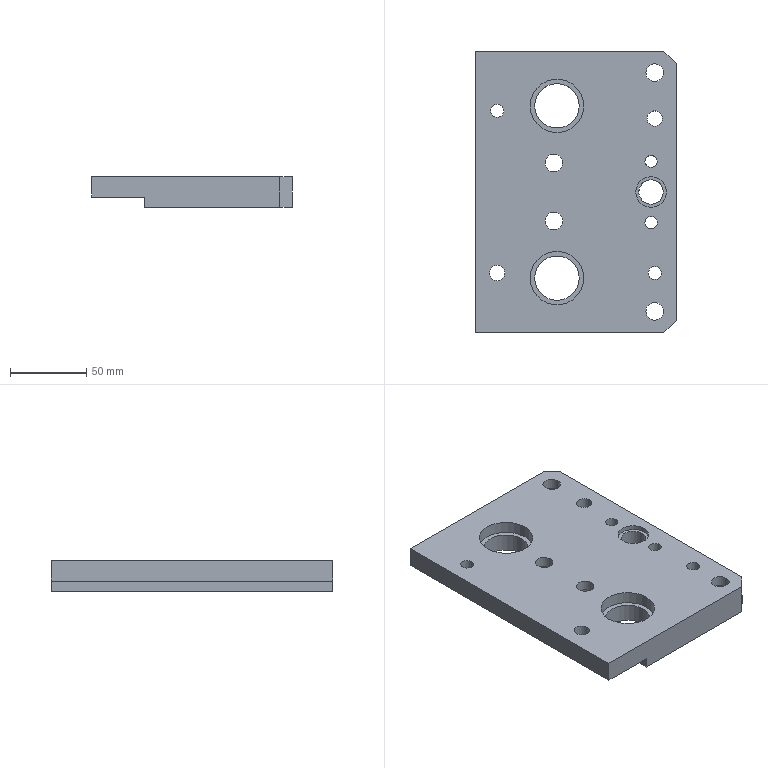Part | STEP file | lll_id3058_x_t | 1 solid | 39 faces | box 131 x 184 x 20 mm | volume 379605 mm3 | cylinder 21 | plane 18 | commonest cylinder face diameters 11.509 x4 18.007 x4 8.505 x2 10 x2 29.07 x2 35 x2
STEP:
#1=CARTESIAN_POINT('',(3278.439,78.,2.5));
#2=VERTEX_POINT('',#1);
#3=CARTESIAN_POINT('',(3269.435,78.,2.5));
#4=DIRECTION('',(0.,0.,1.));
#5=DIRECTION('',(1.,0.,0.));
#6=AXIS2_PLACEMENT_3D('',#3,#4,#5);
#7=CIRCLE('',#6,9.004);
#8=EDGE_CURVE('',#2,#2,#7,.T.);
#9=ORIENTED_EDGE('',*,*,#8,.T.);
#10=EDGE_LOOP('',(#9));
#11=FACE_BOUND('',#10,.T.);
#12=CARTESIAN_POINT('',(3264.435,48.,2.5));
#13=VERTEX_POINT('',#12);
#14=CARTESIAN_POINT('',(3269.435,48.,2.5));
#15=DIRECTION('',(0.,0.,-1.));
#16=DIRECTION('',(-1.,0.,0.));
#17=AXIS2_PLACEMENT_3D('',#14,#15,#16);
#18=CIRCLE('',#17,5.);
#19=EDGE_CURVE('',#13,#13,#18,.T.);
#20=ORIENTED_EDGE('',*,*,#19,.F.);
#21=EDGE_LOOP('',(#20));
#22=FACE_BOUND('',#21,.T.);
#23=CARTESIAN_POINT('',(3267.,16.,2.5));
#24=VERTEX_POINT('',#23);
#25=CARTESIAN_POINT('',(3267.,20.,2.5));
#26=DIRECTION('',(0.,0.,-1.));
#27=DIRECTION('',(0.,-1.,0.));
#28=AXIS2_PLACEMENT_3D('',#25,#26,#27);
#29=CIRCLE('',#28,4.);
#30=EDGE_CURVE('',#24,#24,#29,.T.);
#31=ORIENTED_EDGE('',*,*,#30,.F.);
#32=EDGE_LOOP('',(#31));
#33=FACE_BOUND('',#32,.T.);
#34=CARTESIAN_POINT('',(3267.,-24.05,2.5));
#35=VERTEX_POINT('',#34);
#36=CARTESIAN_POINT('',(3267.,-20.,2.5));
#37=DIRECTION('',(0.,0.,1.));
#38=DIRECTION('',(0.,-1.,0.));
#39=AXIS2_PLACEMENT_3D('',#36,#37,#38);
#40=CIRCLE('',#39,4.05);
#41=EDGE_CURVE('',#35,#35,#40,.T.);
#42=ORIENTED_EDGE('',*,*,#41,.T.);
#43=EDGE_LOOP('',(#42));
#44=FACE_BOUND('',#43,.T.);
#45=CARTESIAN_POINT('',(3190.942,56.288,2.5));
#46=VERTEX_POINT('',#45);
#47=CARTESIAN_POINT('',(3205.477,56.288,2.5));
#48=DIRECTION('',(0.,0.,-1.));
#49=DIRECTION('',(-1.,0.,0.));
#50=AXIS2_PLACEMENT_3D('',#47,#48,#49);
#51=CIRCLE('',#50,14.535);
#52=EDGE_CURVE('',#46,#46,#51,.T.);
#53=ORIENTED_EDGE('',*,*,#52,.F.);
#54=EDGE_LOOP('',(#53));
#55=FACE_BOUND('',#54,.T.);
#56=CARTESIAN_POINT('',(3190.942,-56.288,2.5));
#57=VERTEX_POINT('',#56);
#58=CARTESIAN_POINT('',(3205.477,-56.288,2.5));
#59=DIRECTION('',(0.,0.,-1.));
#60=DIRECTION('',(-1.,0.,0.));
#61=AXIS2_PLACEMENT_3D('',#58,#59,#60);
#62=CIRCLE('',#61,14.535);
#63=EDGE_CURVE('',#57,#57,#62,.T.);
#64=ORIENTED_EDGE('',*,*,#63,.F.);
#65=EDGE_LOOP('',(#64));
#66=FACE_BOUND('',#65,.T.);
#67=CARTESIAN_POINT('',(3267.,-8.,2.5));
#68=VERTEX_POINT('',#67);
#69=CARTESIAN_POINT('',(3267.,0.00005959,2.5));
#70=DIRECTION('',(0.,0.,1.));
#71=DIRECTION('',(0.,-1.,0.));
#72=AXIS2_PLACEMENT_3D('',#69,#70,#71);
#73=CIRCLE('',#72,8.);
#74=EDGE_CURVE('',#68,#68,#73,.T.);
#75=ORIENTED_EDGE('',*,*,#74,.T.);
#76=EDGE_LOOP('',(#75));
#77=FACE_BOUND('',#76,.T.);
#78=CARTESIAN_POINT('',(3278.439,-78.,2.5));
#79=VERTEX_POINT('',#78);
#80=CARTESIAN_POINT('',(3269.435,-78.,2.5));
#81=DIRECTION('',(0.,0.,1.));
#82=DIRECTION('',(1.,0.,0.));
#83=AXIS2_PLACEMENT_3D('',#80,#81,#82);
#84=CIRCLE('',#83,9.004);
#85=EDGE_CURVE('',#79,#79,#84,.T.);
#86=ORIENTED_EDGE('',*,*,#85,.T.);
#87=EDGE_LOOP('',(#86));
#88=FACE_BOUND('',#87,.T.);
#89=CARTESIAN_POINT('',(3186.89,92.,2.5));
#90=VERTEX_POINT('',#89);
#91=CARTESIAN_POINT('',(3275.435,92.,2.5));
#92=VERTEX_POINT('',#91);
#93=CARTESIAN_POINT('',(3227.238,92.,2.5));
#94=DIRECTION('',(1.,0.,0.));
#95=VECTOR('',#94,1.);
#96=LINE('',#93,#95);
#97=EDGE_CURVE('',#90,#92,#96,.T.);
#98=ORIENTED_EDGE('',*,*,#97,.T.);
#99=CARTESIAN_POINT('',(3283.435,84.,2.5));
#100=VERTEX_POINT('',#99);
#101=CARTESIAN_POINT('',(3297.337,70.099,2.5));
#102=DIRECTION('',(0.7071,-0.7071,0.));
#103=VECTOR('',#102,1.);
#104=LINE('',#101,#103);
#105=EDGE_CURVE('',#92,#100,#104,.T.);
#106=ORIENTED_EDGE('',*,*,#105,.T.);
#107=CARTESIAN_POINT('',(3283.435,-84.,2.5));
#108=VERTEX_POINT('',#107);
#109=CARTESIAN_POINT('',(3283.435,0.00007614,2.5));
#110=DIRECTION('',(0.,1.,0.));
#111=VECTOR('',#110,1.);
#112=LINE('',#109,#111);
#113=EDGE_CURVE('',#108,#100,#112,.T.);
#114=ORIENTED_EDGE('',*,*,#113,.F.);
#115=CARTESIAN_POINT('',(3275.435,-92.,2.5));
#116=VERTEX_POINT('',#115);
#117=CARTESIAN_POINT('',(3297.337,-70.098,2.5));
#118=DIRECTION('',(-0.7071,-0.7071,0.));
#119=VECTOR('',#118,1.);
#120=LINE('',#117,#119);
#121=EDGE_CURVE('',#108,#116,#120,.T.);
#122=ORIENTED_EDGE('',*,*,#121,.T.);
#123=CARTESIAN_POINT('',(3186.89,-92.,2.5));
#124=VERTEX_POINT('',#123);
#125=CARTESIAN_POINT('',(3227.238,-92.,2.5));
#126=DIRECTION('',(1.,0.,0.));
#127=VECTOR('',#126,1.);
#128=LINE('',#125,#127);
#129=EDGE_CURVE('',#124,#116,#128,.T.);
#130=ORIENTED_EDGE('',*,*,#129,.F.);
#131=CARTESIAN_POINT('',(3186.89,92.,2.5));
#132=DIRECTION('',(0.,1.,0.));
#133=VECTOR('',#132,1.);
#134=LINE('',#131,#133);
#135=EDGE_CURVE('',#124,#90,#134,.T.);
#136=ORIENTED_EDGE('',*,*,#135,.T.);
#137=EDGE_LOOP('',(#98,#106,#114,#122,#130,#136));
#138=FACE_BOUND('',#137,.T.);
#139=CARTESIAN_POINT('',(3194.432,-19.,2.5));
#140=VERTEX_POINT('',#139);
#141=CARTESIAN_POINT('',(3203.435,-19.,2.5));
#142=DIRECTION('',(0.,0.,-1.));
#143=DIRECTION('',(-1.,0.,0.));
#144=AXIS2_PLACEMENT_3D('',#141,#142,#143);
#145=CIRCLE('',#144,9.004);
#146=EDGE_CURVE('',#140,#140,#145,.T.);
#147=ORIENTED_EDGE('',*,*,#146,.F.);
#148=EDGE_LOOP('',(#147));
#149=FACE_BOUND('',#148,.T.);
#150=CARTESIAN_POINT('',(3194.432,19.,2.5));
#151=VERTEX_POINT('',#150);
#152=CARTESIAN_POINT('',(3203.435,19.,2.5));
#153=DIRECTION('',(0.,0.,-1.));
#154=DIRECTION('',(-1.,0.,0.));
#155=AXIS2_PLACEMENT_3D('',#152,#153,#154);
#156=CIRCLE('',#155,9.004);
#157=EDGE_CURVE('',#151,#151,#156,.T.);
#158=ORIENTED_EDGE('',*,*,#157,.F.);
#159=EDGE_LOOP('',(#158));
#160=FACE_BOUND('',#159,.T.);
#161=CARTESIAN_POINT('',(3275.435,-53.,2.5));
#162=VERTEX_POINT('',#161);
#163=CARTESIAN_POINT('',(3269.435,-53.,2.5));
#164=DIRECTION('',(0.,0.,1.));
#165=DIRECTION('',(1.,0.,0.));
#166=AXIS2_PLACEMENT_3D('',#163,#164,#165);
#167=CIRCLE('',#166,6.);
#168=EDGE_CURVE('',#162,#162,#167,.T.);
#169=ORIENTED_EDGE('',*,*,#168,.T.);
#170=EDGE_LOOP('',(#169));
#171=FACE_BOUND('',#170,.T.);
#172=CARTESIAN_POINT('',(3227.238,0.00007614,2.5));
#173=DIRECTION('',(0.,0.,-1.));
#174=DIRECTION('',(-1.,0.,0.));
#175=AXIS2_PLACEMENT_3D('',#172,#173,#174);
#176=PLANE('',#175);
#177=ADVANCED_FACE('',(#11,#22,#33,#44,#55,#66,#77,#88,#138,#149,#160,#171),#176,.T.);
#178=CARTESIAN_POINT('',(3186.89,-92.,9.209));
#179=VERTEX_POINT('',#178);
#180=CARTESIAN_POINT('',(3186.89,-92.,2.5));
#181=DIRECTION('',(0.,0.,1.));
#182=VECTOR('',#181,1.);
#183=LINE('',#180,#182);
#184=EDGE_CURVE('',#124,#179,#183,.T.);
#185=ORIENTED_EDGE('',*,*,#184,.F.);
#186=ORIENTED_EDGE('',*,*,#129,.T.);
#187=CARTESIAN_POINT('',(3275.435,-92.,22.5));
#188=VERTEX_POINT('',#187);
#189=CARTESIAN_POINT('',(3275.435,-92.,22.5));
#190=DIRECTION('',(0.,0.,1.));
#191=VECTOR('',#190,1.);
#192=LINE('',#189,#191);
#193=EDGE_CURVE('',#116,#188,#192,.T.);
#194=ORIENTED_EDGE('',*,*,#193,.T.);
#195=CARTESIAN_POINT('',(3152.435,-92.,22.5));
#196=VERTEX_POINT('',#195);
#197=CARTESIAN_POINT('',(3227.238,-92.,22.5));
#198=DIRECTION('',(1.,0.,0.));
#199=VECTOR('',#198,1.);
#200=LINE('',#197,#199);
#201=EDGE_CURVE('',#196,#188,#200,.T.);
#202=ORIENTED_EDGE('',*,*,#201,.F.);
#203=CARTESIAN_POINT('',(3152.435,-92.,9.209));
#204=VERTEX_POINT('',#203);
#205=CARTESIAN_POINT('',(3152.435,-92.,27.5));
#206=DIRECTION('',(0.,0.,1.));
#207=VECTOR('',#206,1.);
#208=LINE('',#205,#207);
#209=EDGE_CURVE('',#204,#196,#208,.T.);
#210=ORIENTED_EDGE('',*,*,#209,.F.);
#211=CARTESIAN_POINT('',(3169.662,-92.,9.209));
#212=DIRECTION('',(-1.,0.,0.));
#213=VECTOR('',#212,1.);
#214=LINE('',#211,#213);
#215=EDGE_CURVE('',#179,#204,#214,.T.);
#216=ORIENTED_EDGE('',*,*,#215,.F.);
#217=EDGE_LOOP('',(#185,#186,#194,#202,#210,#216));
#218=FACE_OUTER_BOUND('',#217,.T.);
#219=CARTESIAN_POINT('',(3152.435,-92.,22.5));
#220=DIRECTION('',(0.,1.,0.));
#221=DIRECTION('',(0.,0.,1.));
#222=AXIS2_PLACEMENT_3D('',#219,#220,#221);
#223=PLANE('',#222);
#224=ADVANCED_FACE('',(#218),#223,.F.);
#225=CARTESIAN_POINT('',(3152.435,92.,22.5));
#226=VERTEX_POINT('',#225);
#227=CARTESIAN_POINT('',(3152.435,0.,22.5));
#228=DIRECTION('',(0.,1.,0.));
#229=VECTOR('',#228,1.);
#230=LINE('',#227,#229);
#231=EDGE_CURVE('',#196,#226,#230,.T.);
#232=ORIENTED_EDGE('',*,*,#231,.T.);
#233=CARTESIAN_POINT('',(3152.435,92.,9.209));
#234=VERTEX_POINT('',#233);
#235=CARTESIAN_POINT('',(3152.435,92.,27.5));
#236=DIRECTION('',(0.,0.,-1.));
#237=VECTOR('',#236,1.);
#238=LINE('',#235,#237);
#239=EDGE_CURVE('',#226,#234,#238,.T.);
#240=ORIENTED_EDGE('',*,*,#239,.T.);
#241=CARTESIAN_POINT('',(3152.435,0.,9.209));
#242=DIRECTION('',(0.,1.,0.));
#243=VECTOR('',#242,1.);
#244=LINE('',#241,#243);
#245=EDGE_CURVE('',#204,#234,#244,.T.);
#246=ORIENTED_EDGE('',*,*,#245,.F.);
#247=ORIENTED_EDGE('',*,*,#209,.T.);
#248=EDGE_LOOP('',(#232,#240,#246,#247));
#249=FACE_OUTER_BOUND('',#248,.T.);
#250=CARTESIAN_POINT('',(3152.435,0.,27.5));
#251=DIRECTION('',(-1.,0.,0.));
#252=DIRECTION('',(0.,0.,-1.));
#253=AXIS2_PLACEMENT_3D('',#250,#251,#252);
#254=PLANE('',#253);
#255=ADVANCED_FACE('',(#249),#254,.T.);
#256=CARTESIAN_POINT('',(3209.19,19.,22.5));
#257=VERTEX_POINT('',#256);
#258=CARTESIAN_POINT('',(3203.435,19.,22.5));
#259=DIRECTION('',(0.,0.,1.));
#260=DIRECTION('',(1.,0.,0.));
#261=AXIS2_PLACEMENT_3D('',#258,#259,#260);
#262=CIRCLE('',#261,5.755);
#263=EDGE_CURVE('',#257,#257,#262,.T.);
#264=ORIENTED_EDGE('',*,*,#263,.F.);
#265=EDGE_LOOP('',(#264));
#266=FACE_BOUND('',#265,.T.);
#267=CARTESIAN_POINT('',(3209.19,-19.,22.5));
#268=VERTEX_POINT('',#267);
#269=CARTESIAN_POINT('',(3203.435,-19.,22.5));
#270=DIRECTION('',(0.,0.,1.));
#271=DIRECTION('',(1.,0.,0.));
#272=AXIS2_PLACEMENT_3D('',#269,#270,#271);
#273=CIRCLE('',#272,5.755);
#274=EDGE_CURVE('',#268,#268,#273,.T.);
#275=ORIENTED_EDGE('',*,*,#274,.F.);
#276=EDGE_LOOP('',(#275));
#277=FACE_BOUND('',#276,.T.);
#278=CARTESIAN_POINT('',(3275.19,78.,22.5));
#279=VERTEX_POINT('',#278);
#280=CARTESIAN_POINT('',(3269.435,78.,22.5));
#281=DIRECTION('',(0.,0.,1.));
#282=DIRECTION('',(1.,0.,0.));
#283=AXIS2_PLACEMENT_3D('',#280,#281,#282);
#284=CIRCLE('',#283,5.755);
#285=EDGE_CURVE('',#279,#279,#284,.T.);
#286=ORIENTED_EDGE('',*,*,#285,.F.);
#287=EDGE_LOOP('',(#286));
#288=FACE_BOUND('',#287,.T.);
#289=CARTESIAN_POINT('',(3171.435,-53.,22.5));
#290=VERTEX_POINT('',#289);
#291=CARTESIAN_POINT('',(3166.435,-53.,22.5));
#292=DIRECTION('',(0.,0.,1.));
#293=DIRECTION('',(1.,0.,0.));
#294=AXIS2_PLACEMENT_3D('',#291,#292,#293);
#295=CIRCLE('',#294,5.);
#296=EDGE_CURVE('',#290,#290,#295,.T.);
#297=ORIENTED_EDGE('',*,*,#296,.F.);
#298=EDGE_LOOP('',(#297));
#299=FACE_BOUND('',#298,.T.);
#300=CARTESIAN_POINT('',(3273.688,-53.,22.5));
#301=VERTEX_POINT('',#300);
#302=CARTESIAN_POINT('',(3269.435,-53.,22.5));
#303=DIRECTION('',(0.,0.,1.));
#304=DIRECTION('',(1.,0.,0.));
#305=AXIS2_PLACEMENT_3D('',#302,#303,#304);
#306=CIRCLE('',#305,4.253);
#307=EDGE_CURVE('',#301,#301,#306,.T.);
#308=ORIENTED_EDGE('',*,*,#307,.F.);
#309=EDGE_LOOP('',(#308));
#310=FACE_BOUND('',#309,.T.);
#311=CARTESIAN_POINT('',(3274.435,48.,22.5));
#312=VERTEX_POINT('',#311);
#313=CARTESIAN_POINT('',(3269.435,48.,22.5));
#314=DIRECTION('',(0.,0.,1.));
#315=DIRECTION('',(1.,0.,0.));
#316=AXIS2_PLACEMENT_3D('',#313,#314,#315);
#317=CIRCLE('',#316,5.);
#318=EDGE_CURVE('',#312,#312,#317,.T.);
#319=ORIENTED_EDGE('',*,*,#318,.F.);
#320=EDGE_LOOP('',(#319));
#321=FACE_BOUND('',#320,.T.);
#322=CARTESIAN_POINT('',(3275.19,-78.,22.5));
#323=VERTEX_POINT('',#322);
#324=CARTESIAN_POINT('',(3269.435,-78.,22.5));
#325=DIRECTION('',(0.,0.,1.));
#326=DIRECTION('',(1.,0.,0.));
#327=AXIS2_PLACEMENT_3D('',#324,#325,#326);
#328=CIRCLE('',#327,5.755);
#329=EDGE_CURVE('',#323,#323,#328,.T.);
#330=ORIENTED_EDGE('',*,*,#329,.F.);
#331=EDGE_LOOP('',(#330));
#332=FACE_BOUND('',#331,.T.);
#333=CARTESIAN_POINT('',(3170.688,53.,22.5));
#334=VERTEX_POINT('',#333);
#335=CARTESIAN_POINT('',(3166.435,53.,22.5));
#336=DIRECTION('',(0.,0.,1.));
#337=DIRECTION('',(1.,0.,0.));
#338=AXIS2_PLACEMENT_3D('',#335,#336,#337);
#339=CIRCLE('',#338,4.253);
#340=EDGE_CURVE('',#334,#334,#339,.T.);
#341=ORIENTED_EDGE('',*,*,#340,.F.);
#342=EDGE_LOOP('',(#341));
#343=FACE_BOUND('',#342,.T.);
#344=CARTESIAN_POINT('',(3222.977,56.288,22.5));
#345=VERTEX_POINT('',#344);
#346=CARTESIAN_POINT('',(3205.477,56.288,22.5));
#347=DIRECTION('',(0.,0.,1.));
#348=DIRECTION('',(1.,0.,0.));
#349=AXIS2_PLACEMENT_3D('',#346,#347,#348);
#350=CIRCLE('',#349,17.5);
#351=EDGE_CURVE('',#345,#345,#350,.T.);
#352=ORIENTED_EDGE('',*,*,#351,.F.);
#353=EDGE_LOOP('',(#352));
#354=FACE_BOUND('',#353,.T.);
#355=CARTESIAN_POINT('',(3222.977,-56.288,22.5));
#356=VERTEX_POINT('',#355);
#357=CARTESIAN_POINT('',(3205.477,-56.288,22.5));
#358=DIRECTION('',(0.,0.,1.));
#359=DIRECTION('',(1.,0.,0.));
#360=AXIS2_PLACEMENT_3D('',#357,#358,#359);
#361=CIRCLE('',#360,17.5);
#362=EDGE_CURVE('',#356,#356,#361,.T.);
#363=ORIENTED_EDGE('',*,*,#362,.F.);
#364=EDGE_LOOP('',(#363));
#365=FACE_BOUND('',#364,.T.);
#366=CARTESIAN_POINT('',(3277.,0.00005959,22.5));
#367=VERTEX_POINT('',#366);
#368=CARTESIAN_POINT('',(3267.,0.00005959,22.5));
#369=DIRECTION('',(0.,0.,1.));
#370=DIRECTION('',(1.,0.,0.));
#371=AXIS2_PLACEMENT_3D('',#368,#369,#370);
#372=CIRCLE('',#371,10.);
#373=EDGE_CURVE('',#367,#367,#372,.T.);
#374=ORIENTED_EDGE('',*,*,#373,.F.);
#375=EDGE_LOOP('',(#374));
#376=FACE_BOUND('',#375,.T.);
#377=CARTESIAN_POINT('',(3275.435,92.,22.5));
#378=VERTEX_POINT('',#377);
#379=CARTESIAN_POINT('',(3227.238,92.,22.5));
#380=DIRECTION('',(1.,0.,0.));
#381=VECTOR('',#380,1.);
#382=LINE('',#379,#381);
#383=EDGE_CURVE('',#226,#378,#382,.T.);
#384=ORIENTED_EDGE('',*,*,#383,.F.);
#385=ORIENTED_EDGE('',*,*,#231,.F.);
#386=ORIENTED_EDGE('',*,*,#201,.T.);
#387=CARTESIAN_POINT('',(3283.435,-84.,22.5));
#388=VERTEX_POINT('',#387);
#389=CARTESIAN_POINT('',(3297.337,-70.098,22.5));
#390=DIRECTION('',(0.7071,0.7071,0.));
#391=VECTOR('',#390,1.);
#392=LINE('',#389,#391);
#393=EDGE_CURVE('',#188,#388,#392,.T.);
#394=ORIENTED_EDGE('',*,*,#393,.T.);
#395=CARTESIAN_POINT('',(3283.435,84.,22.5));
#396=VERTEX_POINT('',#395);
#397=CARTESIAN_POINT('',(3283.435,0.00007614,22.5));
#398=DIRECTION('',(0.,-1.,0.));
#399=VECTOR('',#398,1.);
#400=LINE('',#397,#399);
#401=EDGE_CURVE('',#396,#388,#400,.T.);
#402=ORIENTED_EDGE('',*,*,#401,.F.);
#403=CARTESIAN_POINT('',(3297.337,70.099,22.5));
#404=DIRECTION('',(-0.7071,0.7071,0.));
#405=VECTOR('',#404,1.);
#406=LINE('',#403,#405);
#407=EDGE_CURVE('',#396,#378,#406,.T.);
#408=ORIENTED_EDGE('',*,*,#407,.T.);
#409=EDGE_LOOP('',(#384,#385,#386,#394,#402,#408));
#410=FACE_BOUND('',#409,.T.);
#411=CARTESIAN_POINT('',(3271.,20.,22.5));
#412=VERTEX_POINT('',#411);
#413=CARTESIAN_POINT('',(3267.,20.,22.5));
#414=DIRECTION('',(0.,0.,1.));
#415=DIRECTION('',(1.,0.,0.));
#416=AXIS2_PLACEMENT_3D('',#413,#414,#415);
#417=CIRCLE('',#416,4.);
#418=EDGE_CURVE('',#412,#412,#417,.T.);
#419=ORIENTED_EDGE('',*,*,#418,.F.);
#420=EDGE_LOOP('',(#419));
#421=FACE_BOUND('',#420,.T.);
#422=CARTESIAN_POINT('',(3271.05,-20.,22.5));
#423=VERTEX_POINT('',#422);
#424=CARTESIAN_POINT('',(3267.,-20.,22.5));
#425=DIRECTION('',(0.,0.,1.));
#426=DIRECTION('',(1.,0.,0.));
#427=AXIS2_PLACEMENT_3D('',#424,#425,#426);
#428=CIRCLE('',#427,4.05);
#429=EDGE_CURVE('',#423,#423,#428,.T.);
#430=ORIENTED_EDGE('',*,*,#429,.F.);
#431=EDGE_LOOP('',(#430));
#432=FACE_BOUND('',#431,.T.);
#433=CARTESIAN_POINT('',(3227.238,0.00007614,22.5));
#434=DIRECTION('',(0.,0.,1.));
#435=DIRECTION('',(1.,0.,0.));
#436=AXIS2_PLACEMENT_3D('',#433,#434,#435);
#437=PLANE('',#436);
#438=ADVANCED_FACE('',(#266,#277,#288,#299,#310,#321,#332,#343,#354,#365,#376,#410,#421,#432),#437,.T.);
#439=CARTESIAN_POINT('',(3186.89,92.,9.209));
#440=VERTEX_POINT('',#439);
#441=CARTESIAN_POINT('',(3169.662,92.,9.209));
#442=DIRECTION('',(1.,0.,0.));
#443=VECTOR('',#442,1.);
#444=LINE('',#441,#443);
#445=EDGE_CURVE('',#234,#440,#444,.T.);
#446=ORIENTED_EDGE('',*,*,#445,.F.);
#447=ORIENTED_EDGE('',*,*,#239,.F.);
#448=ORIENTED_EDGE('',*,*,#383,.T.);
#449=CARTESIAN_POINT('',(3275.435,92.,2.5));
#450=DIRECTION('',(0.,0.,-1.));
#451=VECTOR('',#450,1.);
#452=LINE('',#449,#451);
#453=EDGE_CURVE('',#378,#92,#452,.T.);
#454=ORIENTED_EDGE('',*,*,#453,.T.);
#455=ORIENTED_EDGE('',*,*,#97,.F.);
#456=CARTESIAN_POINT('',(3186.89,92.,2.5));
#457=DIRECTION('',(0.,0.,1.));
#458=VECTOR('',#457,1.);
#459=LINE('',#456,#458);
#460=EDGE_CURVE('',#90,#440,#459,.T.);
#461=ORIENTED_EDGE('',*,*,#460,.T.);
#462=EDGE_LOOP('',(#446,#447,#448,#454,#455,#461));
#463=FACE_OUTER_BOUND('',#462,.T.);
#464=CARTESIAN_POINT('',(3152.435,92.,22.5));
#465=DIRECTION('',(0.,1.,0.));
#466=DIRECTION('',(0.,0.,1.));
#467=AXIS2_PLACEMENT_3D('',#464,#465,#466);
#468=PLANE('',#467);
#469=ADVANCED_FACE('',(#463),#468,.T.);
#470=CARTESIAN_POINT('',(3275.19,78.,15.5));
#471=VERTEX_POINT('',#470);
#472=CARTESIAN_POINT('',(3269.435,78.,15.5));
#473=DIRECTION('',(0.,0.,1.));
#474=DIRECTION('',(1.,0.,0.));
#475=AXIS2_PLACEMENT_3D('',#472,#473,#474);
#476=CIRCLE('',#475,5.755);
#477=EDGE_CURVE('',#471,#471,#476,.T.);
#478=ORIENTED_EDGE('',*,*,#477,.T.);
#479=EDGE_LOOP('',(#478));
#480=FACE_BOUND('',#479,.T.);
#481=CARTESIAN_POINT('',(3278.439,78.,15.5));
#482=VERTEX_POINT('',#481);
#483=CARTESIAN_POINT('',(3269.435,78.,15.5));
#484=DIRECTION('',(0.,0.,1.));
#485=DIRECTION('',(1.,0.,0.));
#486=AXIS2_PLACEMENT_3D('',#483,#484,#485);
#487=CIRCLE('',#486,9.004);
#488=EDGE_CURVE('',#482,#482,#487,.T.);
#489=ORIENTED_EDGE('',*,*,#488,.F.);
#490=EDGE_LOOP('',(#489));
#491=FACE_BOUND('',#490,.T.);
#492=CARTESIAN_POINT('',(3269.435,78.,15.5));
#493=DIRECTION('',(0.,0.,1.));
#494=DIRECTION('',(1.,0.,0.));
#495=AXIS2_PLACEMENT_3D('',#492,#493,#494);
#496=PLANE('',#495);
#497=ADVANCED_FACE('',(#480,#491),#496,.F.);
#498=CARTESIAN_POINT('',(3222.977,56.288,14.5));
#499=VERTEX_POINT('',#498);
#500=CARTESIAN_POINT('',(3205.477,56.288,14.5));
#501=DIRECTION('',(0.,0.,-1.));
#502=DIRECTION('',(1.,0.,0.));
#503=AXIS2_PLACEMENT_3D('',#500,#501,#502);
#504=CIRCLE('',#503,17.5);
#505=EDGE_CURVE('',#499,#499,#504,.T.);
#506=ORIENTED_EDGE('',*,*,#505,.F.);
#507=EDGE_LOOP('',(#506));
#508=FACE_BOUND('',#507,.T.);
#509=CARTESIAN_POINT('',(3220.012,56.288,14.5));
#510=VERTEX_POINT('',#509);
#511=CARTESIAN_POINT('',(3205.477,56.288,14.5));
#512=DIRECTION('',(0.,0.,-1.));
#513=DIRECTION('',(1.,0.,0.));
#514=AXIS2_PLACEMENT_3D('',#511,#512,#513);
#515=CIRCLE('',#514,14.535);
#516=EDGE_CURVE('',#510,#510,#515,.T.);
#517=ORIENTED_EDGE('',*,*,#516,.T.);
#518=EDGE_LOOP('',(#517));
#519=FACE_BOUND('',#518,.T.);
#520=CARTESIAN_POINT('',(3205.477,56.288,14.5));
#521=DIRECTION('',(0.,0.,1.));
#522=DIRECTION('',(1.,0.,0.));
#523=AXIS2_PLACEMENT_3D('',#520,#521,#522);
#524=PLANE('',#523);
#525=ADVANCED_FACE('',(#508,#519),#524,.T.);
#526=CARTESIAN_POINT('',(3222.977,-56.288,14.5));
#527=VERTEX_POINT('',#526);
#528=CARTESIAN_POINT('',(3205.477,-56.288,14.5));
#529=DIRECTION('',(0.,0.,-1.));
#530=DIRECTION('',(1.,0.,0.));
#531=AXIS2_PLACEMENT_3D('',#528,#529,#530);
#532=CIRCLE('',#531,17.5);
#533=EDGE_CURVE('',#527,#527,#532,.T.);
#534=ORIENTED_EDGE('',*,*,#533,.F.);
#535=EDGE_LOOP('',(#534));
#536=FACE_BOUND('',#535,.T.);
#537=CARTESIAN_POINT('',(3220.012,-56.288,14.5));
#538=VERTEX_POINT('',#537);
#539=CARTESIAN_POINT('',(3205.477,-56.288,14.5));
#540=DIRECTION('',(0.,0.,-1.));
#541=DIRECTION('',(1.,0.,0.));
#542=AXIS2_PLACEMENT_3D('',#539,#540,#541);
#543=CIRCLE('',#542,14.535);
#544=EDGE_CURVE('',#538,#538,#543,.T.);
#545=ORIENTED_EDGE('',*,*,#544,.T.);
#546=EDGE_LOOP('',(#545));
#547=FACE_BOUND('',#546,.T.);
#548=CARTESIAN_POINT('',(3205.477,-56.288,14.5));
#549=DIRECTION('',(0.,0.,1.));
#550=DIRECTION('',(1.,0.,0.));
#551=AXIS2_PLACEMENT_3D('',#548,#549,#550);
#552=PLANE('',#551);
#553=ADVANCED_FACE('',(#536,#547),#552,.T.);
#554=CARTESIAN_POINT('',(3257.,0.00005959,19.5));
#555=VERTEX_POINT('',#554);
#556=CARTESIAN_POINT('',(3267.,0.00005959,19.5));
#557=DIRECTION('',(0.,0.,1.));
#558=DIRECTION('',(-1.,0.,0.));
#559=AXIS2_PLACEMENT_3D('',#556,#557,#558);
#560=CIRCLE('',#559,10.);
#561=EDGE_CURVE('',#555,#555,#560,.T.);
#562=ORIENTED_EDGE('',*,*,#561,.T.);
#563=EDGE_LOOP('',(#562));
#564=FACE_BOUND('',#563,.T.);
#565=CARTESIAN_POINT('',(3259.,0.00005959,19.5));
#566=VERTEX_POINT('',#565);
#567=CARTESIAN_POINT('',(3267.,0.00005959,19.5));
#568=DIRECTION('',(0.,0.,1.));
#569=DIRECTION('',(-1.,0.,0.));
#570=AXIS2_PLACEMENT_3D('',#567,#568,#569);
#571=CIRCLE('',#570,8.);
#572=EDGE_CURVE('',#566,#566,#571,.T.);
#573=ORIENTED_EDGE('',*,*,#572,.F.);
#574=EDGE_LOOP('',(#573));
#575=FACE_BOUND('',#574,.T.);
#576=CARTESIAN_POINT('',(3267.,0.00005959,19.5));
#577=DIRECTION('',(0.,0.,-1.));
#578=DIRECTION('',(0.,1.,0.));
#579=AXIS2_PLACEMENT_3D('',#576,#577,#578);
#580=PLANE('',#579);
#581=ADVANCED_FACE('',(#564,#575),#580,.F.);
#582=CARTESIAN_POINT('',(3275.19,-78.,15.5));
#583=VERTEX_POINT('',#582);
#584=CARTESIAN_POINT('',(3269.435,-78.,15.5));
#585=DIRECTION('',(0.,0.,1.));
#586=DIRECTION('',(1.,0.,0.));
#587=AXIS2_PLACEMENT_3D('',#584,#585,#586);
#588=CIRCLE('',#587,5.755);
#589=EDGE_CURVE('',#583,#583,#588,.T.);
#590=ORIENTED_EDGE('',*,*,#589,.T.);
#591=EDGE_LOOP('',(#590));
#592=FACE_BOUND('',#591,.T.);
#593=CARTESIAN_POINT('',(3278.439,-78.,15.5));
#594=VERTEX_POINT('',#593);
#595=CARTESIAN_POINT('',(3269.435,-78.,15.5));
#596=DIRECTION('',(0.,0.,1.));
#597=DIRECTION('',(1.,0.,0.));
#598=AXIS2_PLACEMENT_3D('',#595,#596,#597);
#599=CIRCLE('',#598,9.004);
#600=EDGE_CURVE('',#594,#594,#599,.T.);
#601=ORIENTED_EDGE('',*,*,#600,.F.);
#602=EDGE_LOOP('',(#601));
#603=FACE_BOUND('',#602,.T.);
#604=CARTESIAN_POINT('',(3269.435,-78.,15.5));
#605=DIRECTION('',(0.,0.,1.));
#606=DIRECTION('',(1.,0.,0.));
#607=AXIS2_PLACEMENT_3D('',#604,#605,#606);
#608=PLANE('',#607);
#609=ADVANCED_FACE('',(#592,#603),#608,.F.);
#610=CARTESIAN_POINT('',(3209.19,-19.,15.5));
#611=VERTEX_POINT('',#610);
#612=CARTESIAN_POINT('',(3203.435,-19.,15.5));
#613=DIRECTION('',(0.,0.,1.));
#614=DIRECTION('',(1.,0.,0.));
#615=AXIS2_PLACEMENT_3D('',#612,#613,#614);
#616=CIRCLE('',#615,5.755);
#617=EDGE_CURVE('',#611,#611,#616,.T.);
#618=ORIENTED_EDGE('',*,*,#617,.T.);
#619=EDGE_LOOP('',(#618));
#620=FACE_BOUND('',#619,.T.);
#621=CARTESIAN_POINT('',(3212.439,-19.,15.5));
#622=VERTEX_POINT('',#621);
#623=CARTESIAN_POINT('',(3203.435,-19.,15.5));
#624=DIRECTION('',(0.,0.,1.));
#625=DIRECTION('',(1.,0.,0.));
#626=AXIS2_PLACEMENT_3D('',#623,#624,#625);
#627=CIRCLE('',#626,9.004);
#628=EDGE_CURVE('',#622,#622,#627,.T.);
#629=ORIENTED_EDGE('',*,*,#628,.F.);
#630=EDGE_LOOP('',(#629));
#631=FACE_BOUND('',#630,.T.);
#632=CARTESIAN_POINT('',(3203.435,-23.,15.5));
#633=DIRECTION('',(0.,0.,1.));
#634=DIRECTION('',(1.,0.,0.));
#635=AXIS2_PLACEMENT_3D('',#632,#633,#634);
#636=PLANE('',#635);
#637=ADVANCED_FACE('',(#620,#631),#636,.F.);
#638=ORIENTED_EDGE('',*,*,#561,.F.);
#639=EDGE_LOOP('',(#638));
#640=FACE_BOUND('',#639,.T.);
#641=ORIENTED_EDGE('',*,*,#373,.T.);
#642=EDGE_LOOP('',(#641));
#643=FACE_BOUND('',#642,.T.);
#644=CARTESIAN_POINT('',(3267.,0.00005959,17.5));
#645=DIRECTION('',(0.,0.,-1.));
#646=DIRECTION('',(0.,1.,0.));
#647=AXIS2_PLACEMENT_3D('',#644,#645,#646);
#648=CYLINDRICAL_SURFACE('',#647,10.);
#649=ADVANCED_FACE('',(#640,#643),#648,.F.);
#650=ORIENTED_EDGE('',*,*,#362,.T.);
#651=EDGE_LOOP('',(#650));
#652=FACE_BOUND('',#651,.T.);
#653=ORIENTED_EDGE('',*,*,#533,.T.);
#654=EDGE_LOOP('',(#653));
#655=FACE_BOUND('',#654,.T.);
#656=CARTESIAN_POINT('',(3205.477,-56.288,14.5));
#657=DIRECTION('',(0.,0.,1.));
#658=DIRECTION('',(1.,0.,0.));
#659=AXIS2_PLACEMENT_3D('',#656,#657,#658);
#660=CYLINDRICAL_SURFACE('',#659,17.5);
#661=ADVANCED_FACE('',(#652,#655),#660,.F.);
#662=ORIENTED_EDGE('',*,*,#351,.T.);
#663=EDGE_LOOP('',(#662));
#664=FACE_BOUND('',#663,.T.);
#665=ORIENTED_EDGE('',*,*,#505,.T.);
#666=EDGE_LOOP('',(#665));
#667=FACE_BOUND('',#666,.T.);
#668=CARTESIAN_POINT('',(3205.477,56.288,14.5));
#669=DIRECTION('',(0.,0.,1.));
#670=DIRECTION('',(1.,0.,0.));
#671=AXIS2_PLACEMENT_3D('',#668,#669,#670);
#672=CYLINDRICAL_SURFACE('',#671,17.5);
#673=ADVANCED_FACE('',(#664,#667),#672,.F.);
#674=CARTESIAN_POINT('',(3170.688,53.,9.209));
#675=VERTEX_POINT('',#674);
#676=CARTESIAN_POINT('',(3166.435,53.,9.209));
#677=DIRECTION('',(0.,0.,-1.));
#678=DIRECTION('',(1.,0.,0.));
#679=AXIS2_PLACEMENT_3D('',#676,#677,#678);
#680=CIRCLE('',#679,4.253);
#681=EDGE_CURVE('',#675,#675,#680,.T.);
#682=ORIENTED_EDGE('',*,*,#681,.T.);
#683=EDGE_LOOP('',(#682));
#684=FACE_BOUND('',#683,.T.);
#685=ORIENTED_EDGE('',*,*,#340,.T.);
#686=EDGE_LOOP('',(#685));
#687=FACE_BOUND('',#686,.T.);
#688=CARTESIAN_POINT('',(3166.435,53.,-2.5));
#689=DIRECTION('',(0.,0.,1.));
#690=DIRECTION('',(1.,0.,0.));
#691=AXIS2_PLACEMENT_3D('',#688,#689,#690);
#692=CYLINDRICAL_SURFACE('',#691,4.253);
#693=ADVANCED_FACE('',(#684,#687),#692,.F.);
#694=ORIENTED_EDGE('',*,*,#329,.T.);
#695=EDGE_LOOP('',(#694));
#696=FACE_BOUND('',#695,.T.);
#697=ORIENTED_EDGE('',*,*,#589,.F.);
#698=EDGE_LOOP('',(#697));
#699=FACE_BOUND('',#698,.T.);
#700=CARTESIAN_POINT('',(3269.435,-78.,-2.5));
#701=DIRECTION('',(0.,0.,1.));
#702=DIRECTION('',(1.,0.,0.));
#703=AXIS2_PLACEMENT_3D('',#700,#701,#702);
#704=CYLINDRICAL_SURFACE('',#703,5.755);
#705=ADVANCED_FACE('',(#696,#699),#704,.F.);
#706=ORIENTED_EDGE('',*,*,#488,.T.);
#707=EDGE_LOOP('',(#706));
#708=FACE_BOUND('',#707,.T.);
#709=ORIENTED_EDGE('',*,*,#8,.F.);
#710=EDGE_LOOP('',(#709));
#711=FACE_BOUND('',#710,.T.);
#712=CARTESIAN_POINT('',(3269.435,78.,2.5));
#713=DIRECTION('',(0.,0.,1.));
#714=DIRECTION('',(1.,0.,0.));
#715=AXIS2_PLACEMENT_3D('',#712,#713,#714);
#716=CYLINDRICAL_SURFACE('',#715,9.004);
#717=ADVANCED_FACE('',(#708,#711),#716,.F.);
#718=CARTESIAN_POINT('',(3273.688,-53.,7.5));
#719=VERTEX_POINT('',#718);
#720=CARTESIAN_POINT('',(3269.435,-53.,7.5));
#721=DIRECTION('',(0.,0.,-1.));
#722=DIRECTION('',(1.,0.,0.));
#723=AXIS2_PLACEMENT_3D('',#720,#721,#722);
#724=CIRCLE('',#723,4.253);
#725=EDGE_CURVE('',#719,#719,#724,.T.);
#726=ORIENTED_EDGE('',*,*,#725,.T.);
#727=EDGE_LOOP('',(#726));
#728=FACE_BOUND('',#727,.T.);
#729=ORIENTED_EDGE('',*,*,#307,.T.);
#730=EDGE_LOOP('',(#729));
#731=FACE_BOUND('',#730,.T.);
#732=CARTESIAN_POINT('',(3269.435,-53.,-2.5));
#733=DIRECTION('',(0.,0.,1.));
#734=DIRECTION('',(1.,0.,0.));
#735=AXIS2_PLACEMENT_3D('',#732,#733,#734);
#736=CYLINDRICAL_SURFACE('',#735,4.253);
#737=ADVANCED_FACE('',(#728,#731),#736,.F.);
#738=ORIENTED_EDGE('',*,*,#19,.T.);
#739=EDGE_LOOP('',(#738));
#740=FACE_BOUND('',#739,.T.);
#741=ORIENTED_EDGE('',*,*,#318,.T.);
#742=EDGE_LOOP('',(#741));
#743=FACE_BOUND('',#742,.T.);
#744=CARTESIAN_POINT('',(3269.435,48.,-2.5));
#745=DIRECTION('',(0.,0.,1.));
#746=DIRECTION('',(1.,0.,0.));
#747=AXIS2_PLACEMENT_3D('',#744,#745,#746);
#748=CYLINDRICAL_SURFACE('',#747,5.);
#749=ADVANCED_FACE('',(#740,#743),#748,.F.);
#750=ORIENTED_EDGE('',*,*,#418,.T.);
#751=EDGE_LOOP('',(#750));
#752=FACE_BOUND('',#751,.T.);
#753=ORIENTED_EDGE('',*,*,#30,.T.);
#754=EDGE_LOOP('',(#753));
#755=FACE_BOUND('',#754,.T.);
#756=CARTESIAN_POINT('',(3267.,20.,-40.259));
#757=DIRECTION('',(0.,0.,1.));
#758=DIRECTION('',(-1.,0.,0.));
#759=AXIS2_PLACEMENT_3D('',#756,#757,#758);
#760=CYLINDRICAL_SURFACE('',#759,4.);
#761=ADVANCED_FACE('',(#752,#755),#760,.F.);
#762=ORIENTED_EDGE('',*,*,#41,.F.);
#763=EDGE_LOOP('',(#762));
#764=FACE_BOUND('',#763,.T.);
#765=ORIENTED_EDGE('',*,*,#429,.T.);
#766=EDGE_LOOP('',(#765));
#767=FACE_BOUND('',#766,.T.);
#768=CARTESIAN_POINT('',(3267.,-20.,-40.259));
#769=DIRECTION('',(0.,0.,1.));
#770=DIRECTION('',(1.,0.,0.));
#771=AXIS2_PLACEMENT_3D('',#768,#769,#770);
#772=CYLINDRICAL_SURFACE('',#771,4.05);
#773=ADVANCED_FACE('',(#764,#767),#772,.F.);
#774=ORIENTED_EDGE('',*,*,#52,.T.);
#775=EDGE_LOOP('',(#774));
#776=FACE_BOUND('',#775,.T.);
#777=ORIENTED_EDGE('',*,*,#516,.F.);
#778=EDGE_LOOP('',(#777));
#779=FACE_BOUND('',#778,.T.);
#780=CARTESIAN_POINT('',(3205.477,56.288,5.));
#781=DIRECTION('',(0.,0.,-1.));
#782=DIRECTION('',(-1.,0.,0.));
#783=AXIS2_PLACEMENT_3D('',#780,#781,#782);
#784=CYLINDRICAL_SURFACE('',#783,14.535);
#785=ADVANCED_FACE('',(#776,#779),#784,.F.);
#786=ORIENTED_EDGE('',*,*,#63,.T.);
#787=EDGE_LOOP('',(#786));
#788=FACE_BOUND('',#787,.T.);
#789=ORIENTED_EDGE('',*,*,#544,.F.);
#790=EDGE_LOOP('',(#789));
#791=FACE_BOUND('',#790,.T.);
#792=CARTESIAN_POINT('',(3205.477,-56.288,5.));
#793=DIRECTION('',(0.,0.,-1.));
#794=DIRECTION('',(-1.,0.,0.));
#795=AXIS2_PLACEMENT_3D('',#792,#793,#794);
#796=CYLINDRICAL_SURFACE('',#795,14.535);
#797=ADVANCED_FACE('',(#788,#791),#796,.F.);
#798=ORIENTED_EDGE('',*,*,#572,.T.);
#799=EDGE_LOOP('',(#798));
#800=FACE_BOUND('',#799,.T.);
#801=ORIENTED_EDGE('',*,*,#74,.F.);
#802=EDGE_LOOP('',(#801));
#803=FACE_BOUND('',#802,.T.);
#804=CARTESIAN_POINT('',(3267.,0.00005959,25.));
#805=DIRECTION('',(0.,0.,-1.));
#806=DIRECTION('',(0.,1.,0.));
#807=AXIS2_PLACEMENT_3D('',#804,#805,#806);
#808=CYLINDRICAL_SURFACE('',#807,8.);
#809=ADVANCED_FACE('',(#800,#803),#808,.F.);
#810=ORIENTED_EDGE('',*,*,#600,.T.);
#811=EDGE_LOOP('',(#810));
#812=FACE_BOUND('',#811,.T.);
#813=ORIENTED_EDGE('',*,*,#85,.F.);
#814=EDGE_LOOP('',(#813));
#815=FACE_BOUND('',#814,.T.);
#816=CARTESIAN_POINT('',(3269.435,-78.,2.5));
#817=DIRECTION('',(0.,0.,1.));
#818=DIRECTION('',(1.,0.,0.));
#819=AXIS2_PLACEMENT_3D('',#816,#817,#818);
#820=CYLINDRICAL_SURFACE('',#819,9.004);
#821=ADVANCED_FACE('',(#812,#815),#820,.F.);
#822=ORIENTED_EDGE('',*,*,#113,.T.);
#823=CARTESIAN_POINT('',(3283.435,84.,22.5));
#824=DIRECTION('',(0.,0.,1.));
#825=VECTOR('',#824,1.);
#826=LINE('',#823,#825);
#827=EDGE_CURVE('',#100,#396,#826,.T.);
#828=ORIENTED_EDGE('',*,*,#827,.T.);
#829=ORIENTED_EDGE('',*,*,#401,.T.);
#830=CARTESIAN_POINT('',(3283.435,-84.,12.5));
#831=DIRECTION('',(0.,0.,-1.));
#832=VECTOR('',#831,1.);
#833=LINE('',#830,#832);
#834=EDGE_CURVE('',#388,#108,#833,.T.);
#835=ORIENTED_EDGE('',*,*,#834,.T.);
#836=EDGE_LOOP('',(#822,#828,#829,#835));
#837=FACE_OUTER_BOUND('',#836,.T.);
#838=CARTESIAN_POINT('',(3283.435,0.00007614,12.5));
#839=DIRECTION('',(-1.,0.,0.));
#840=DIRECTION('',(0.,0.,1.));
#841=AXIS2_PLACEMENT_3D('',#838,#839,#840);
#842=PLANE('',#841);
#843=ADVANCED_FACE('',(#837),#842,.F.);
#844=ORIENTED_EDGE('',*,*,#628,.T.);
#845=EDGE_LOOP('',(#844));
#846=FACE_BOUND('',#845,.T.);
#847=ORIENTED_EDGE('',*,*,#146,.T.);
#848=EDGE_LOOP('',(#847));
#849=FACE_BOUND('',#848,.T.);
#850=CARTESIAN_POINT('',(3203.435,-19.,2.5));
#851=DIRECTION('',(0.,0.,1.));
#852=DIRECTION('',(1.,0.,0.));
#853=AXIS2_PLACEMENT_3D('',#850,#851,#852);
#854=CYLINDRICAL_SURFACE('',#853,9.004);
#855=ADVANCED_FACE('',(#846,#849),#854,.F.);
#856=CARTESIAN_POINT('',(3171.435,-53.,9.209));
#857=VERTEX_POINT('',#856);
#858=CARTESIAN_POINT('',(3166.435,-53.,9.209));
#859=DIRECTION('',(0.,0.,-1.));
#860=DIRECTION('',(1.,0.,0.));
#861=AXIS2_PLACEMENT_3D('',#858,#859,#860);
#862=CIRCLE('',#861,5.);
#863=EDGE_CURVE('',#857,#857,#862,.T.);
#864=ORIENTED_EDGE('',*,*,#863,.T.);
#865=EDGE_LOOP('',(#864));
#866=FACE_BOUND('',#865,.T.);
#867=ORIENTED_EDGE('',*,*,#296,.T.);
#868=EDGE_LOOP('',(#867));
#869=FACE_BOUND('',#868,.T.);
#870=CARTESIAN_POINT('',(3166.435,-53.,-2.5));
#871=DIRECTION('',(0.,0.,1.));
#872=DIRECTION('',(1.,0.,0.));
#873=AXIS2_PLACEMENT_3D('',#870,#871,#872);
#874=CYLINDRICAL_SURFACE('',#873,5.);
#875=ADVANCED_FACE('',(#866,#869),#874,.F.);
#876=ORIENTED_EDGE('',*,*,#285,.T.);
#877=EDGE_LOOP('',(#876));
#878=FACE_BOUND('',#877,.T.);
#879=ORIENTED_EDGE('',*,*,#477,.F.);
#880=EDGE_LOOP('',(#879));
#881=FACE_BOUND('',#880,.T.);
#882=CARTESIAN_POINT('',(3269.435,78.,-2.5));
#883=DIRECTION('',(0.,0.,1.));
#884=DIRECTION('',(1.,0.,0.));
#885=AXIS2_PLACEMENT_3D('',#882,#883,#884);
#886=CYLINDRICAL_SURFACE('',#885,5.755);
#887=ADVANCED_FACE('',(#878,#881),#886,.F.);
#888=ORIENTED_EDGE('',*,*,#274,.T.);
#889=EDGE_LOOP('',(#888));
#890=FACE_BOUND('',#889,.T.);
#891=ORIENTED_EDGE('',*,*,#617,.F.);
#892=EDGE_LOOP('',(#891));
#893=FACE_BOUND('',#892,.T.);
#894=CARTESIAN_POINT('',(3203.435,-19.,-2.5));
#895=DIRECTION('',(0.,0.,1.));
#896=DIRECTION('',(1.,0.,0.));
#897=AXIS2_PLACEMENT_3D('',#894,#895,#896);
#898=CYLINDRICAL_SURFACE('',#897,5.755);
#899=ADVANCED_FACE('',(#890,#893),#898,.F.);
#900=CARTESIAN_POINT('',(3209.19,19.,15.5));
#901=VERTEX_POINT('',#900);
#902=CARTESIAN_POINT('',(3203.435,19.,15.5));
#903=DIRECTION('',(0.,0.,1.));
#904=DIRECTION('',(1.,0.,0.));
#905=AXIS2_PLACEMENT_3D('',#902,#903,#904);
#906=CIRCLE('',#905,5.755);
#907=EDGE_CURVE('',#901,#901,#906,.T.);
#908=ORIENTED_EDGE('',*,*,#907,.T.);
#909=EDGE_LOOP('',(#908));
#910=FACE_BOUND('',#909,.T.);
#911=CARTESIAN_POINT('',(3212.439,19.,15.5));
#912=VERTEX_POINT('',#911);
#913=CARTESIAN_POINT('',(3203.435,19.,15.5));
#914=DIRECTION('',(0.,0.,1.));
#915=DIRECTION('',(1.,0.,0.));
#916=AXIS2_PLACEMENT_3D('',#913,#914,#915);
#917=CIRCLE('',#916,9.004);
#918=EDGE_CURVE('',#912,#912,#917,.T.);
#919=ORIENTED_EDGE('',*,*,#918,.F.);
#920=EDGE_LOOP('',(#919));
#921=FACE_BOUND('',#920,.T.);
#922=CARTESIAN_POINT('',(3203.435,7.,15.5));
#923=DIRECTION('',(0.,0.,1.));
#924=DIRECTION('',(1.,0.,0.));
#925=AXIS2_PLACEMENT_3D('',#922,#923,#924);
#926=PLANE('',#925);
#927=ADVANCED_FACE('',(#910,#921),#926,.F.);
#928=ORIENTED_EDGE('',*,*,#918,.T.);
#929=EDGE_LOOP('',(#928));
#930=FACE_BOUND('',#929,.T.);
#931=ORIENTED_EDGE('',*,*,#157,.T.);
#932=EDGE_LOOP('',(#931));
#933=FACE_BOUND('',#932,.T.);
#934=CARTESIAN_POINT('',(3203.435,19.,2.5));
#935=DIRECTION('',(0.,0.,1.));
#936=DIRECTION('',(1.,0.,0.));
#937=AXIS2_PLACEMENT_3D('',#934,#935,#936);
#938=CYLINDRICAL_SURFACE('',#937,9.004);
#939=ADVANCED_FACE('',(#930,#933),#938,.F.);
#940=ORIENTED_EDGE('',*,*,#263,.T.);
#941=EDGE_LOOP('',(#940));
#942=FACE_BOUND('',#941,.T.);
#943=ORIENTED_EDGE('',*,*,#907,.F.);
#944=EDGE_LOOP('',(#943));
#945=FACE_BOUND('',#944,.T.);
#946=CARTESIAN_POINT('',(3203.435,19.,-2.5));
#947=DIRECTION('',(0.,0.,1.));
#948=DIRECTION('',(1.,0.,0.));
#949=AXIS2_PLACEMENT_3D('',#946,#947,#948);
#950=CYLINDRICAL_SURFACE('',#949,5.755);
#951=ADVANCED_FACE('',(#942,#945),#950,.F.);
#952=ORIENTED_EDGE('',*,*,#407,.F.);
#953=ORIENTED_EDGE('',*,*,#827,.F.);
#954=ORIENTED_EDGE('',*,*,#105,.F.);
#955=ORIENTED_EDGE('',*,*,#453,.F.);
#956=EDGE_LOOP('',(#952,#953,#954,#955));
#957=FACE_OUTER_BOUND('',#956,.T.);
#958=CARTESIAN_POINT('',(3275.435,92.,22.5));
#959=DIRECTION('',(0.7071,0.7071,0.));
#960=DIRECTION('',(0.,0.,1.));
#961=AXIS2_PLACEMENT_3D('',#958,#959,#960);
#962=PLANE('',#961);
#963=ADVANCED_FACE('',(#957),#962,.T.);
#964=ORIENTED_EDGE('',*,*,#121,.F.);
#965=ORIENTED_EDGE('',*,*,#834,.F.);
#966=ORIENTED_EDGE('',*,*,#393,.F.);
#967=ORIENTED_EDGE('',*,*,#193,.F.);
#968=EDGE_LOOP('',(#964,#965,#966,#967));
#969=FACE_OUTER_BOUND('',#968,.T.);
#970=CARTESIAN_POINT('',(3275.435,-92.,22.5));
#971=DIRECTION('',(-0.7071,0.7071,0.));
#972=DIRECTION('',(0.,0.,1.));
#973=AXIS2_PLACEMENT_3D('',#970,#971,#972);
#974=PLANE('',#973);
#975=ADVANCED_FACE('',(#969),#974,.F.);
#976=ORIENTED_EDGE('',*,*,#863,.F.);
#977=EDGE_LOOP('',(#976));
#978=FACE_BOUND('',#977,.T.);
#979=ORIENTED_EDGE('',*,*,#215,.T.);
#980=ORIENTED_EDGE('',*,*,#245,.T.);
#981=ORIENTED_EDGE('',*,*,#445,.T.);
#982=CARTESIAN_POINT('',(3186.89,0.00007614,9.209));
#983=DIRECTION('',(0.,1.,0.));
#984=VECTOR('',#983,1.);
#985=LINE('',#982,#984);
#986=EDGE_CURVE('',#179,#440,#985,.T.);
#987=ORIENTED_EDGE('',*,*,#986,.F.);
#988=EDGE_LOOP('',(#979,#980,#981,#987));
#989=FACE_BOUND('',#988,.T.);
#990=ORIENTED_EDGE('',*,*,#681,.F.);
#991=EDGE_LOOP('',(#990));
#992=FACE_BOUND('',#991,.T.);
#993=CARTESIAN_POINT('',(3169.662,0.00007614,9.209));
#994=DIRECTION('',(0.,0.,1.));
#995=DIRECTION('',(1.,0.,0.));
#996=AXIS2_PLACEMENT_3D('',#993,#994,#995);
#997=PLANE('',#996);
#998=ADVANCED_FACE('',(#978,#989,#992),#997,.F.);
#999=ORIENTED_EDGE('',*,*,#135,.F.);
#1000=ORIENTED_EDGE('',*,*,#184,.T.);
#1001=ORIENTED_EDGE('',*,*,#986,.T.);
#1002=ORIENTED_EDGE('',*,*,#460,.F.);
#1003=EDGE_LOOP('',(#999,#1000,#1001,#1002));
#1004=FACE_OUTER_BOUND('',#1003,.T.);
#1005=CARTESIAN_POINT('',(3186.89,0.00007614,2.5));
#1006=DIRECTION('',(1.,0.,0.));
#1007=DIRECTION('',(0.,0.,-1.));
#1008=AXIS2_PLACEMENT_3D('',#1005,#1006,#1007);
#1009=PLANE('',#1008);
#1010=ADVANCED_FACE('',(#1004),#1009,.F.);
#1011=CARTESIAN_POINT('',(3275.435,-53.,7.5));
#1012=VERTEX_POINT('',#1011);
#1013=CARTESIAN_POINT('',(3269.435,-53.,7.5));
#1014=DIRECTION('',(0.,0.,1.));
#1015=DIRECTION('',(1.,0.,0.));
#1016=AXIS2_PLACEMENT_3D('',#1013,#1014,#1015);
#1017=CIRCLE('',#1016,6.);
#1018=EDGE_CURVE('',#1012,#1012,#1017,.T.);
#1019=ORIENTED_EDGE('',*,*,#1018,.F.);
#1020=EDGE_LOOP('',(#1019));
#1021=FACE_BOUND('',#1020,.T.);
#1022=ORIENTED_EDGE('',*,*,#725,.F.);
#1023=EDGE_LOOP('',(#1022));
#1024=FACE_BOUND('',#1023,.T.);
#1025=CARTESIAN_POINT('',(3269.435,-53.,7.5));
#1026=DIRECTION('',(0.,0.,1.));
#1027=DIRECTION('',(1.,0.,0.));
#1028=AXIS2_PLACEMENT_3D('',#1025,#1026,#1027);
#1029=PLANE('',#1028);
#1030=ADVANCED_FACE('',(#1021,#1024),#1029,.F.);
#1031=ORIENTED_EDGE('',*,*,#1018,.T.);
#1032=EDGE_LOOP('',(#1031));
#1033=FACE_BOUND('',#1032,.T.);
#1034=ORIENTED_EDGE('',*,*,#168,.F.);
#1035=EDGE_LOOP('',(#1034));
#1036=FACE_BOUND('',#1035,.T.);
#1037=CARTESIAN_POINT('',(3269.435,-53.,2.5));
#1038=DIRECTION('',(0.,0.,1.));
#1039=DIRECTION('',(1.,0.,0.));
#1040=AXIS2_PLACEMENT_3D('',#1037,#1038,#1039);
#1041=CYLINDRICAL_SURFACE('',#1040,6.);
#1042=ADVANCED_FACE('',(#1033,#1036),#1041,.F.);
#1043=CLOSED_SHELL('',(#177,#224,#255,#438,#469,#497,#525,#553,#581,#609,#637,#649,#661,#673,#693,#705,#717,#737,#749,#761,#773,#785,#797,#809,#821,#843,#855,#875,#887,#899,#927,#939,#951,#963,#975,#998,#1010,#1030,#1042));
#1044=MANIFOLD_SOLID_BREP('',#1043);
#1045=(LENGTH_UNIT()NAMED_UNIT(*)SI_UNIT(.MILLI.,.METRE.));
#1046=UNCERTAINTY_MEASURE_WITH_UNIT(LENGTH_MEASURE(0.00002),#1045,'','');
#1047=(NAMED_UNIT(*)PLANE_ANGLE_UNIT()SI_UNIT($,.RADIAN.));
#1048=PLANE_ANGLE_MEASURE_WITH_UNIT(PLANE_ANGLE_MEASURE(0.01745),#1047);
#1049=DIMENSIONAL_EXPONENTS(0.,0.,0.,0.,0.,0.,0.);
#1050=(CONVERSION_BASED_UNIT('DEGREE',#1048)NAMED_UNIT(#1049)PLANE_ANGLE_UNIT());
#1051=(NAMED_UNIT(*)SI_UNIT($,.STERADIAN.)SOLID_ANGLE_UNIT());
#1052=(GEOMETRIC_REPRESENTATION_CONTEXT(3)GLOBAL_UNCERTAINTY_ASSIGNED_CONTEXT((#1046))GLOBAL_UNIT_ASSIGNED_CONTEXT((#1045,#1050,#1051))REPRESENTATION_CONTEXT('',''));
#1053=ADVANCED_BREP_SHAPE_REPRESENTATION('',(#1044),#1052);